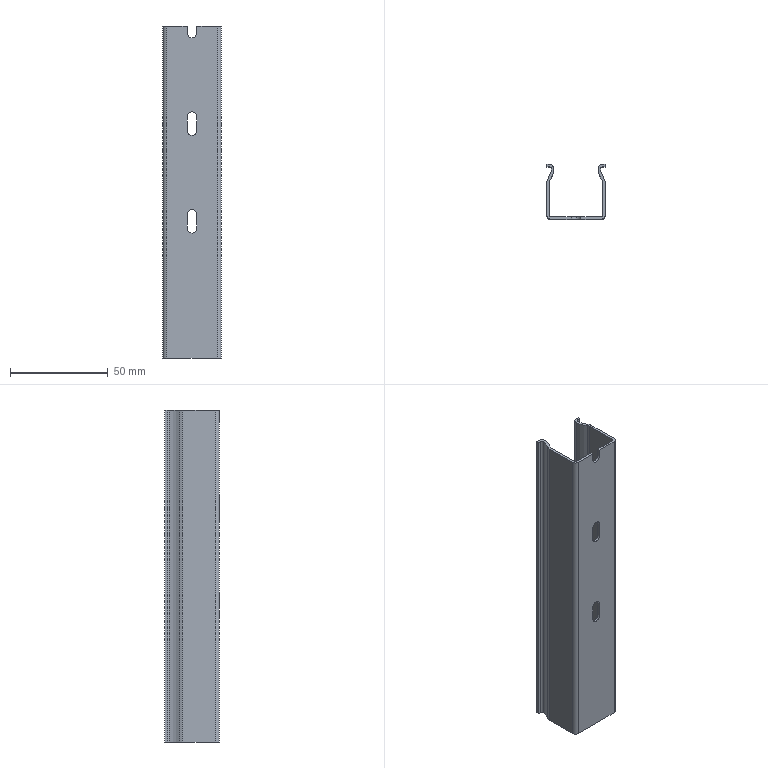Part | SolidWorks | features BaseBody 1 | 1 solid | 47 faces | box 30 x 28 x 170 mm | volume 18284 mm3 | cylinder 26 | plane 21 | commonest cylinder face diameters 5 x8 2 x3 4.5 x3 1.5 x2 3.5 x2 4 x2
STEP:
#1=CARTESIAN_POINT('',(-2.5,-12.75,-103.5));
#2=VERTEX_POINT('',#1);
#3=CARTESIAN_POINT('',(-2.5,-12.75,-96.5));
#4=VERTEX_POINT('',#3);
#5=CARTESIAN_POINT('',(-2.5,-12.75,-96.5));
#6=DIRECTION('',(0.,0.,1.));
#7=VECTOR('',#6,1000.);
#8=LINE('',#5,#7);
#9=EDGE_CURVE('',#2,#4,#8,.T.);
#10=ORIENTED_EDGE('',*,*,#9,.T.);
#11=CARTESIAN_POINT('',(-2.5,-14.,-96.5));
#12=VERTEX_POINT('',#11);
#13=CARTESIAN_POINT('',(-2.5,14.001,-96.5));
#14=DIRECTION('',(0.,-1.,0.));
#15=VECTOR('',#14,1000.);
#16=LINE('',#13,#15);
#17=EDGE_CURVE('',#4,#12,#16,.T.);
#18=ORIENTED_EDGE('',*,*,#17,.T.);
#19=CARTESIAN_POINT('',(-2.5,-14.,-103.5));
#20=VERTEX_POINT('',#19);
#21=CARTESIAN_POINT('',(-2.5,-14.,-96.5));
#22=DIRECTION('',(0.,0.,-1.));
#23=VECTOR('',#22,1000.);
#24=LINE('',#21,#23);
#25=EDGE_CURVE('',#12,#20,#24,.T.);
#26=ORIENTED_EDGE('',*,*,#25,.T.);
#27=CARTESIAN_POINT('',(-2.5,14.001,-103.5));
#28=DIRECTION('',(0.,-1.,0.));
#29=VECTOR('',#28,1000.);
#30=LINE('',#27,#29);
#31=EDGE_CURVE('',#2,#20,#30,.T.);
#32=ORIENTED_EDGE('',*,*,#31,.F.);
#33=EDGE_LOOP('',(#10,#18,#26,#32));
#34=FACE_OUTER_BOUND('',#33,.T.);
#35=CARTESIAN_POINT('',(-2.5,14.001,-96.5));
#36=DIRECTION('',(-1.,0.,0.));
#37=DIRECTION('',(0.,0.,1.));
#38=AXIS2_PLACEMENT_3D('',#35,#36,#37);
#39=PLANE('',#38);
#40=ADVANCED_FACE('',(#34),#39,.F.);
#41=CARTESIAN_POINT('',(0.,-12.75,-106.));
#42=VERTEX_POINT('',#41);
#43=CARTESIAN_POINT('',(0.,-14.,-106.));
#44=VERTEX_POINT('',#43);
#45=CARTESIAN_POINT('',(0.,14.001,-106.));
#46=DIRECTION('',(0.,-1.,0.));
#47=VECTOR('',#46,1000.);
#48=LINE('',#45,#47);
#49=EDGE_CURVE('',#42,#44,#48,.T.);
#50=ORIENTED_EDGE('',*,*,#49,.F.);
#51=CARTESIAN_POINT('',(0.,-12.75,-103.5));
#52=DIRECTION('',(0.,1.,0.));
#53=DIRECTION('',(0.,0.,-1.));
#54=AXIS2_PLACEMENT_3D('',#51,#52,#53);
#55=CIRCLE('',#54,2.5);
#56=EDGE_CURVE('',#42,#2,#55,.T.);
#57=ORIENTED_EDGE('',*,*,#56,.T.);
#58=ORIENTED_EDGE('',*,*,#31,.T.);
#59=CARTESIAN_POINT('',(0.,-14.,-103.5));
#60=DIRECTION('',(0.,-1.,0.));
#61=DIRECTION('',(0.,0.,-1.));
#62=AXIS2_PLACEMENT_3D('',#59,#60,#61);
#63=CIRCLE('',#62,2.5);
#64=EDGE_CURVE('',#20,#44,#63,.T.);
#65=ORIENTED_EDGE('',*,*,#64,.T.);
#66=EDGE_LOOP('',(#50,#57,#58,#65));
#67=FACE_OUTER_BOUND('',#66,.T.);
#68=CARTESIAN_POINT('',(0.,14.001,-103.5));
#69=DIRECTION('',(0.,-1.,0.));
#70=DIRECTION('',(0.,0.,-1.));
#71=AXIS2_PLACEMENT_3D('',#68,#69,#70);
#72=CYLINDRICAL_SURFACE('',#71,2.5);
#73=ADVANCED_FACE('',(#67),#72,.F.);
#74=CARTESIAN_POINT('',(2.5,-12.75,-96.5));
#75=VERTEX_POINT('',#74);
#76=CARTESIAN_POINT('',(2.5,-12.75,-103.5));
#77=VERTEX_POINT('',#76);
#78=CARTESIAN_POINT('',(2.5,-12.75,-96.5));
#79=DIRECTION('',(0.,0.,-1.));
#80=VECTOR('',#79,1000.);
#81=LINE('',#78,#80);
#82=EDGE_CURVE('',#75,#77,#81,.T.);
#83=ORIENTED_EDGE('',*,*,#82,.T.);
#84=CARTESIAN_POINT('',(2.5,-14.,-103.5));
#85=VERTEX_POINT('',#84);
#86=CARTESIAN_POINT('',(2.5,14.001,-103.5));
#87=DIRECTION('',(0.,-1.,0.));
#88=VECTOR('',#87,1000.);
#89=LINE('',#86,#88);
#90=EDGE_CURVE('',#77,#85,#89,.T.);
#91=ORIENTED_EDGE('',*,*,#90,.T.);
#92=CARTESIAN_POINT('',(2.5,-14.,-96.5));
#93=VERTEX_POINT('',#92);
#94=CARTESIAN_POINT('',(2.5,-14.,-96.5));
#95=DIRECTION('',(0.,0.,1.));
#96=VECTOR('',#95,1000.);
#97=LINE('',#94,#96);
#98=EDGE_CURVE('',#85,#93,#97,.T.);
#99=ORIENTED_EDGE('',*,*,#98,.T.);
#100=CARTESIAN_POINT('',(2.5,14.001,-96.5));
#101=DIRECTION('',(0.,-1.,0.));
#102=VECTOR('',#101,1000.);
#103=LINE('',#100,#102);
#104=EDGE_CURVE('',#75,#93,#103,.T.);
#105=ORIENTED_EDGE('',*,*,#104,.F.);
#106=EDGE_LOOP('',(#83,#91,#99,#105));
#107=FACE_OUTER_BOUND('',#106,.T.);
#108=CARTESIAN_POINT('',(2.5,14.001,-96.5));
#109=DIRECTION('',(1.,0.,0.));
#110=DIRECTION('',(0.,0.,1.));
#111=AXIS2_PLACEMENT_3D('',#108,#109,#110);
#112=PLANE('',#111);
#113=ADVANCED_FACE('',(#107),#112,.F.);
#114=CARTESIAN_POINT('',(0.,-12.75,-96.5));
#115=DIRECTION('',(0.,1.,0.));
#116=DIRECTION('',(0.,0.,-1.));
#117=AXIS2_PLACEMENT_3D('',#114,#115,#116);
#118=CIRCLE('',#117,2.5);
#119=EDGE_CURVE('',#4,#75,#118,.T.);
#120=ORIENTED_EDGE('',*,*,#119,.T.);
#121=ORIENTED_EDGE('',*,*,#104,.T.);
#122=CARTESIAN_POINT('',(0.,-14.,-96.5));
#123=DIRECTION('',(0.,-1.,0.));
#124=DIRECTION('',(0.,0.,-1.));
#125=AXIS2_PLACEMENT_3D('',#122,#123,#124);
#126=CIRCLE('',#125,2.5);
#127=EDGE_CURVE('',#93,#12,#126,.T.);
#128=ORIENTED_EDGE('',*,*,#127,.T.);
#129=ORIENTED_EDGE('',*,*,#17,.F.);
#130=EDGE_LOOP('',(#120,#121,#128,#129));
#131=FACE_OUTER_BOUND('',#130,.T.);
#132=CARTESIAN_POINT('',(0.,14.001,-96.5));
#133=DIRECTION('',(0.,-1.,0.));
#134=DIRECTION('',(0.,0.,-1.));
#135=AXIS2_PLACEMENT_3D('',#132,#133,#134);
#136=CYLINDRICAL_SURFACE('',#135,2.5);
#137=ADVANCED_FACE('',(#131),#136,.F.);
#138=CARTESIAN_POINT('',(-2.5,-12.75,-53.5));
#139=VERTEX_POINT('',#138);
#140=CARTESIAN_POINT('',(-2.5,-12.75,-46.5));
#141=VERTEX_POINT('',#140);
#142=CARTESIAN_POINT('',(-2.5,-12.75,-46.5));
#143=DIRECTION('',(0.,0.,1.));
#144=VECTOR('',#143,1000.);
#145=LINE('',#142,#144);
#146=EDGE_CURVE('',#139,#141,#145,.T.);
#147=ORIENTED_EDGE('',*,*,#146,.T.);
#148=CARTESIAN_POINT('',(-2.5,-14.,-46.5));
#149=VERTEX_POINT('',#148);
#150=CARTESIAN_POINT('',(-2.5,14.001,-46.5));
#151=DIRECTION('',(0.,-1.,0.));
#152=VECTOR('',#151,1000.);
#153=LINE('',#150,#152);
#154=EDGE_CURVE('',#141,#149,#153,.T.);
#155=ORIENTED_EDGE('',*,*,#154,.T.);
#156=CARTESIAN_POINT('',(-2.5,-14.,-53.5));
#157=VERTEX_POINT('',#156);
#158=CARTESIAN_POINT('',(-2.5,-14.,-46.5));
#159=DIRECTION('',(0.,0.,-1.));
#160=VECTOR('',#159,1000.);
#161=LINE('',#158,#160);
#162=EDGE_CURVE('',#149,#157,#161,.T.);
#163=ORIENTED_EDGE('',*,*,#162,.T.);
#164=CARTESIAN_POINT('',(-2.5,14.001,-53.5));
#165=DIRECTION('',(0.,-1.,0.));
#166=VECTOR('',#165,1000.);
#167=LINE('',#164,#166);
#168=EDGE_CURVE('',#139,#157,#167,.T.);
#169=ORIENTED_EDGE('',*,*,#168,.F.);
#170=EDGE_LOOP('',(#147,#155,#163,#169));
#171=FACE_OUTER_BOUND('',#170,.T.);
#172=CARTESIAN_POINT('',(-2.5,14.001,-46.5));
#173=DIRECTION('',(-1.,0.,0.));
#174=DIRECTION('',(0.,0.,1.));
#175=AXIS2_PLACEMENT_3D('',#172,#173,#174);
#176=PLANE('',#175);
#177=ADVANCED_FACE('',(#171),#176,.F.);
#178=CARTESIAN_POINT('',(0.,-12.75,-56.));
#179=VERTEX_POINT('',#178);
#180=CARTESIAN_POINT('',(0.,-14.,-56.));
#181=VERTEX_POINT('',#180);
#182=CARTESIAN_POINT('',(0.,14.001,-56.));
#183=DIRECTION('',(0.,-1.,0.));
#184=VECTOR('',#183,1000.);
#185=LINE('',#182,#184);
#186=EDGE_CURVE('',#179,#181,#185,.T.);
#187=ORIENTED_EDGE('',*,*,#186,.F.);
#188=CARTESIAN_POINT('',(0.,-12.75,-53.5));
#189=DIRECTION('',(0.,1.,0.));
#190=DIRECTION('',(0.,0.,-1.));
#191=AXIS2_PLACEMENT_3D('',#188,#189,#190);
#192=CIRCLE('',#191,2.5);
#193=EDGE_CURVE('',#179,#139,#192,.T.);
#194=ORIENTED_EDGE('',*,*,#193,.T.);
#195=ORIENTED_EDGE('',*,*,#168,.T.);
#196=CARTESIAN_POINT('',(0.,-14.,-53.5));
#197=DIRECTION('',(0.,-1.,0.));
#198=DIRECTION('',(0.,0.,-1.));
#199=AXIS2_PLACEMENT_3D('',#196,#197,#198);
#200=CIRCLE('',#199,2.5);
#201=EDGE_CURVE('',#157,#181,#200,.T.);
#202=ORIENTED_EDGE('',*,*,#201,.T.);
#203=EDGE_LOOP('',(#187,#194,#195,#202));
#204=FACE_OUTER_BOUND('',#203,.T.);
#205=CARTESIAN_POINT('',(0.,14.001,-53.5));
#206=DIRECTION('',(0.,-1.,0.));
#207=DIRECTION('',(0.,0.,-1.));
#208=AXIS2_PLACEMENT_3D('',#205,#206,#207);
#209=CYLINDRICAL_SURFACE('',#208,2.5);
#210=ADVANCED_FACE('',(#204),#209,.F.);
#211=CARTESIAN_POINT('',(2.5,-12.75,-46.5));
#212=VERTEX_POINT('',#211);
#213=CARTESIAN_POINT('',(2.5,-12.75,-53.5));
#214=VERTEX_POINT('',#213);
#215=CARTESIAN_POINT('',(2.5,-12.75,-46.5));
#216=DIRECTION('',(0.,0.,-1.));
#217=VECTOR('',#216,1000.);
#218=LINE('',#215,#217);
#219=EDGE_CURVE('',#212,#214,#218,.T.);
#220=ORIENTED_EDGE('',*,*,#219,.T.);
#221=CARTESIAN_POINT('',(2.5,-14.,-53.5));
#222=VERTEX_POINT('',#221);
#223=CARTESIAN_POINT('',(2.5,14.001,-53.5));
#224=DIRECTION('',(0.,-1.,0.));
#225=VECTOR('',#224,1000.);
#226=LINE('',#223,#225);
#227=EDGE_CURVE('',#214,#222,#226,.T.);
#228=ORIENTED_EDGE('',*,*,#227,.T.);
#229=CARTESIAN_POINT('',(2.5,-14.,-46.5));
#230=VERTEX_POINT('',#229);
#231=CARTESIAN_POINT('',(2.5,-14.,-46.5));
#232=DIRECTION('',(0.,0.,1.));
#233=VECTOR('',#232,1000.);
#234=LINE('',#231,#233);
#235=EDGE_CURVE('',#222,#230,#234,.T.);
#236=ORIENTED_EDGE('',*,*,#235,.T.);
#237=CARTESIAN_POINT('',(2.5,14.001,-46.5));
#238=DIRECTION('',(0.,-1.,0.));
#239=VECTOR('',#238,1000.);
#240=LINE('',#237,#239);
#241=EDGE_CURVE('',#212,#230,#240,.T.);
#242=ORIENTED_EDGE('',*,*,#241,.F.);
#243=EDGE_LOOP('',(#220,#228,#236,#242));
#244=FACE_OUTER_BOUND('',#243,.T.);
#245=CARTESIAN_POINT('',(2.5,14.001,-46.5));
#246=DIRECTION('',(1.,0.,0.));
#247=DIRECTION('',(0.,0.,1.));
#248=AXIS2_PLACEMENT_3D('',#245,#246,#247);
#249=PLANE('',#248);
#250=ADVANCED_FACE('',(#244),#249,.F.);
#251=CARTESIAN_POINT('',(0.,-12.75,-46.5));
#252=DIRECTION('',(0.,1.,0.));
#253=DIRECTION('',(0.,0.,-1.));
#254=AXIS2_PLACEMENT_3D('',#251,#252,#253);
#255=CIRCLE('',#254,2.5);
#256=EDGE_CURVE('',#141,#212,#255,.T.);
#257=ORIENTED_EDGE('',*,*,#256,.T.);
#258=ORIENTED_EDGE('',*,*,#241,.T.);
#259=CARTESIAN_POINT('',(0.,-14.,-46.5));
#260=DIRECTION('',(0.,-1.,0.));
#261=DIRECTION('',(0.,0.,-1.));
#262=AXIS2_PLACEMENT_3D('',#259,#260,#261);
#263=CIRCLE('',#262,2.5);
#264=EDGE_CURVE('',#230,#149,#263,.T.);
#265=ORIENTED_EDGE('',*,*,#264,.T.);
#266=ORIENTED_EDGE('',*,*,#154,.F.);
#267=EDGE_LOOP('',(#257,#258,#265,#266));
#268=FACE_OUTER_BOUND('',#267,.T.);
#269=CARTESIAN_POINT('',(0.,14.001,-46.5));
#270=DIRECTION('',(0.,-1.,0.));
#271=DIRECTION('',(0.,0.,-1.));
#272=AXIS2_PLACEMENT_3D('',#269,#270,#271);
#273=CYLINDRICAL_SURFACE('',#272,2.5);
#274=ADVANCED_FACE('',(#268),#273,.F.);
#275=CARTESIAN_POINT('',(-2.5,-14.,0.));
#276=VERTEX_POINT('',#275);
#277=CARTESIAN_POINT('',(-2.5,-14.,-3.5));
#278=VERTEX_POINT('',#277);
#279=CARTESIAN_POINT('',(-2.5,-14.,3.5));
#280=DIRECTION('',(0.,0.,-1.));
#281=VECTOR('',#280,1000.);
#282=LINE('',#279,#281);
#283=EDGE_CURVE('',#276,#278,#282,.T.);
#284=ORIENTED_EDGE('',*,*,#283,.T.);
#285=CARTESIAN_POINT('',(-2.5,-12.75,-3.5));
#286=VERTEX_POINT('',#285);
#287=CARTESIAN_POINT('',(-2.5,14.001,-3.5));
#288=DIRECTION('',(0.,-1.,0.));
#289=VECTOR('',#288,1000.);
#290=LINE('',#287,#289);
#291=EDGE_CURVE('',#286,#278,#290,.T.);
#292=ORIENTED_EDGE('',*,*,#291,.F.);
#293=CARTESIAN_POINT('',(-2.5,-12.75,0.));
#294=VERTEX_POINT('',#293);
#295=CARTESIAN_POINT('',(-2.5,-12.75,3.5));
#296=DIRECTION('',(0.,0.,1.));
#297=VECTOR('',#296,1000.);
#298=LINE('',#295,#297);
#299=EDGE_CURVE('',#286,#294,#298,.T.);
#300=ORIENTED_EDGE('',*,*,#299,.T.);
#301=CARTESIAN_POINT('',(-2.5,14.001,0.));
#302=DIRECTION('',(0.,1.,0.));
#303=VECTOR('',#302,1000.);
#304=LINE('',#301,#303);
#305=EDGE_CURVE('',#276,#294,#304,.T.);
#306=ORIENTED_EDGE('',*,*,#305,.F.);
#307=EDGE_LOOP('',(#284,#292,#300,#306));
#308=FACE_OUTER_BOUND('',#307,.T.);
#309=CARTESIAN_POINT('',(-2.5,14.001,3.5));
#310=DIRECTION('',(-1.,0.,0.));
#311=DIRECTION('',(0.,0.,1.));
#312=AXIS2_PLACEMENT_3D('',#309,#310,#311);
#313=PLANE('',#312);
#314=ADVANCED_FACE('',(#308),#313,.F.);
#315=CARTESIAN_POINT('',(2.5,-12.75,0.));
#316=VERTEX_POINT('',#315);
#317=CARTESIAN_POINT('',(2.5,-12.75,-3.5));
#318=VERTEX_POINT('',#317);
#319=CARTESIAN_POINT('',(2.5,-12.75,3.5));
#320=DIRECTION('',(0.,0.,-1.));
#321=VECTOR('',#320,1000.);
#322=LINE('',#319,#321);
#323=EDGE_CURVE('',#316,#318,#322,.T.);
#324=ORIENTED_EDGE('',*,*,#323,.T.);
#325=CARTESIAN_POINT('',(2.5,-14.,-3.5));
#326=VERTEX_POINT('',#325);
#327=CARTESIAN_POINT('',(2.5,14.001,-3.5));
#328=DIRECTION('',(0.,-1.,0.));
#329=VECTOR('',#328,1000.);
#330=LINE('',#327,#329);
#331=EDGE_CURVE('',#318,#326,#330,.T.);
#332=ORIENTED_EDGE('',*,*,#331,.T.);
#333=CARTESIAN_POINT('',(2.5,-14.,0.));
#334=VERTEX_POINT('',#333);
#335=CARTESIAN_POINT('',(2.5,-14.,3.5));
#336=DIRECTION('',(0.,0.,1.));
#337=VECTOR('',#336,1000.);
#338=LINE('',#335,#337);
#339=EDGE_CURVE('',#326,#334,#338,.T.);
#340=ORIENTED_EDGE('',*,*,#339,.T.);
#341=CARTESIAN_POINT('',(2.5,14.001,0.));
#342=DIRECTION('',(0.,-1.,0.));
#343=VECTOR('',#342,1000.);
#344=LINE('',#341,#343);
#345=EDGE_CURVE('',#316,#334,#344,.T.);
#346=ORIENTED_EDGE('',*,*,#345,.F.);
#347=EDGE_LOOP('',(#324,#332,#340,#346));
#348=FACE_OUTER_BOUND('',#347,.T.);
#349=CARTESIAN_POINT('',(2.5,14.001,3.5));
#350=DIRECTION('',(1.,0.,0.));
#351=DIRECTION('',(0.,0.,1.));
#352=AXIS2_PLACEMENT_3D('',#349,#350,#351);
#353=PLANE('',#352);
#354=ADVANCED_FACE('',(#348),#353,.F.);
#355=CARTESIAN_POINT('',(0.,-12.75,-6.));
#356=VERTEX_POINT('',#355);
#357=CARTESIAN_POINT('',(0.,-14.,-6.));
#358=VERTEX_POINT('',#357);
#359=CARTESIAN_POINT('',(0.,14.001,-6.));
#360=DIRECTION('',(0.,-1.,0.));
#361=VECTOR('',#360,1000.);
#362=LINE('',#359,#361);
#363=EDGE_CURVE('',#356,#358,#362,.T.);
#364=ORIENTED_EDGE('',*,*,#363,.F.);
#365=CARTESIAN_POINT('',(0.,-12.75,-3.5));
#366=DIRECTION('',(0.,1.,0.));
#367=DIRECTION('',(0.,0.,-1.));
#368=AXIS2_PLACEMENT_3D('',#365,#366,#367);
#369=CIRCLE('',#368,2.5);
#370=EDGE_CURVE('',#356,#286,#369,.T.);
#371=ORIENTED_EDGE('',*,*,#370,.T.);
#372=ORIENTED_EDGE('',*,*,#291,.T.);
#373=CARTESIAN_POINT('',(0.,-14.,-3.5));
#374=DIRECTION('',(0.,-1.,0.));
#375=DIRECTION('',(0.,0.,-1.));
#376=AXIS2_PLACEMENT_3D('',#373,#374,#375);
#377=CIRCLE('',#376,2.5);
#378=EDGE_CURVE('',#278,#358,#377,.T.);
#379=ORIENTED_EDGE('',*,*,#378,.T.);
#380=EDGE_LOOP('',(#364,#371,#372,#379));
#381=FACE_OUTER_BOUND('',#380,.T.);
#382=CARTESIAN_POINT('',(0.,14.001,-3.5));
#383=DIRECTION('',(0.,-1.,0.));
#384=DIRECTION('',(0.,0.,-1.));
#385=AXIS2_PLACEMENT_3D('',#382,#383,#384);
#386=CYLINDRICAL_SURFACE('',#385,2.5);
#387=ADVANCED_FACE('',(#381),#386,.F.);
#388=CARTESIAN_POINT('',(-13.,-12.75,-170.));
#389=VERTEX_POINT('',#388);
#390=CARTESIAN_POINT('',(-13.75,-12.,-170.));
#391=VERTEX_POINT('',#390);
#392=CARTESIAN_POINT('',(-13.,-12.,-170.));
#393=DIRECTION('',(0.,0.,-1.));
#394=DIRECTION('',(1.,0.,0.));
#395=AXIS2_PLACEMENT_3D('',#392,#393,#394);
#396=CIRCLE('',#395,0.75);
#397=EDGE_CURVE('',#389,#391,#396,.T.);
#398=ORIENTED_EDGE('',*,*,#397,.T.);
#399=CARTESIAN_POINT('',(-13.75,-12.,0.));
#400=VERTEX_POINT('',#399);
#401=CARTESIAN_POINT('',(-13.75,-12.,-170.));
#402=DIRECTION('',(0.,0.,1.));
#403=VECTOR('',#402,1000.);
#404=LINE('',#401,#403);
#405=EDGE_CURVE('',#391,#400,#404,.T.);
#406=ORIENTED_EDGE('',*,*,#405,.T.);
#407=CARTESIAN_POINT('',(-13.,-12.75,0.));
#408=VERTEX_POINT('',#407);
#409=CARTESIAN_POINT('',(-13.,-12.,0.));
#410=DIRECTION('',(0.,0.,1.));
#411=DIRECTION('',(1.,0.,0.));
#412=AXIS2_PLACEMENT_3D('',#409,#410,#411);
#413=CIRCLE('',#412,0.75);
#414=EDGE_CURVE('',#400,#408,#413,.T.);
#415=ORIENTED_EDGE('',*,*,#414,.T.);
#416=CARTESIAN_POINT('',(-13.,-12.75,-170.));
#417=DIRECTION('',(0.,0.,-1.));
#418=VECTOR('',#417,1000.);
#419=LINE('',#416,#418);
#420=EDGE_CURVE('',#408,#389,#419,.T.);
#421=ORIENTED_EDGE('',*,*,#420,.T.);
#422=EDGE_LOOP('',(#398,#406,#415,#421));
#423=FACE_OUTER_BOUND('',#422,.T.);
#424=CARTESIAN_POINT('',(-13.,-12.,-170.));
#425=DIRECTION('',(0.,0.,1.));
#426=DIRECTION('',(1.,0.,0.));
#427=AXIS2_PLACEMENT_3D('',#424,#425,#426);
#428=CYLINDRICAL_SURFACE('',#427,0.75);
#429=ADVANCED_FACE('',(#423),#428,.F.);
#430=CARTESIAN_POINT('',(13.75,-12.,-170.));
#431=VERTEX_POINT('',#430);
#432=CARTESIAN_POINT('',(13.,-12.75,-170.));
#433=VERTEX_POINT('',#432);
#434=CARTESIAN_POINT('',(13.,-12.,-170.));
#435=DIRECTION('',(0.,0.,-1.));
#436=DIRECTION('',(1.,0.,0.));
#437=AXIS2_PLACEMENT_3D('',#434,#435,#436);
#438=CIRCLE('',#437,0.75);
#439=EDGE_CURVE('',#431,#433,#438,.T.);
#440=ORIENTED_EDGE('',*,*,#439,.T.);
#441=CARTESIAN_POINT('',(13.,-12.75,0.));
#442=VERTEX_POINT('',#441);
#443=CARTESIAN_POINT('',(13.,-12.75,-170.));
#444=DIRECTION('',(0.,0.,1.));
#445=VECTOR('',#444,1000.);
#446=LINE('',#443,#445);
#447=EDGE_CURVE('',#433,#442,#446,.T.);
#448=ORIENTED_EDGE('',*,*,#447,.T.);
#449=CARTESIAN_POINT('',(13.75,-12.,0.));
#450=VERTEX_POINT('',#449);
#451=CARTESIAN_POINT('',(13.,-12.,0.));
#452=DIRECTION('',(0.,0.,1.));
#453=DIRECTION('',(1.,0.,0.));
#454=AXIS2_PLACEMENT_3D('',#451,#452,#453);
#455=CIRCLE('',#454,0.75);
#456=EDGE_CURVE('',#442,#450,#455,.T.);
#457=ORIENTED_EDGE('',*,*,#456,.T.);
#458=CARTESIAN_POINT('',(13.75,-12.,-170.));
#459=DIRECTION('',(0.,0.,-1.));
#460=VECTOR('',#459,1000.);
#461=LINE('',#458,#460);
#462=EDGE_CURVE('',#450,#431,#461,.T.);
#463=ORIENTED_EDGE('',*,*,#462,.T.);
#464=EDGE_LOOP('',(#440,#448,#457,#463));
#465=FACE_OUTER_BOUND('',#464,.T.);
#466=CARTESIAN_POINT('',(13.,-12.,-170.));
#467=DIRECTION('',(0.,0.,1.));
#468=DIRECTION('',(1.,0.,0.));
#469=AXIS2_PLACEMENT_3D('',#466,#467,#468);
#470=CYLINDRICAL_SURFACE('',#469,0.75);
#471=ADVANCED_FACE('',(#465),#470,.F.);
#472=CARTESIAN_POINT('',(13.439,5.746,-170.));
#473=VERTEX_POINT('',#472);
#474=CARTESIAN_POINT('',(13.75,4.75,-170.));
#475=VERTEX_POINT('',#474);
#476=CARTESIAN_POINT('',(12.,4.75,-170.));
#477=DIRECTION('',(0.,0.,-1.));
#478=DIRECTION('',(1.,0.,0.));
#479=AXIS2_PLACEMENT_3D('',#476,#477,#478);
#480=CIRCLE('',#479,1.75);
#481=EDGE_CURVE('',#473,#475,#480,.T.);
#482=ORIENTED_EDGE('',*,*,#481,.T.);
#483=CARTESIAN_POINT('',(13.75,4.75,0.));
#484=VERTEX_POINT('',#483);
#485=CARTESIAN_POINT('',(13.75,4.75,-170.));
#486=DIRECTION('',(0.,0.,1.));
#487=VECTOR('',#486,1000.);
#488=LINE('',#485,#487);
#489=EDGE_CURVE('',#475,#484,#488,.T.);
#490=ORIENTED_EDGE('',*,*,#489,.T.);
#491=CARTESIAN_POINT('',(13.439,5.746,0.));
#492=VERTEX_POINT('',#491);
#493=CARTESIAN_POINT('',(12.,4.75,0.));
#494=DIRECTION('',(0.,0.,1.));
#495=DIRECTION('',(1.,0.,0.));
#496=AXIS2_PLACEMENT_3D('',#493,#494,#495);
#497=CIRCLE('',#496,1.75);
#498=EDGE_CURVE('',#484,#492,#497,.T.);
#499=ORIENTED_EDGE('',*,*,#498,.T.);
#500=CARTESIAN_POINT('',(13.439,5.746,-170.));
#501=DIRECTION('',(0.,0.,-1.));
#502=VECTOR('',#501,1000.);
#503=LINE('',#500,#502);
#504=EDGE_CURVE('',#492,#473,#503,.T.);
#505=ORIENTED_EDGE('',*,*,#504,.T.);
#506=EDGE_LOOP('',(#482,#490,#499,#505));
#507=FACE_OUTER_BOUND('',#506,.T.);
#508=CARTESIAN_POINT('',(12.,4.75,-170.));
#509=DIRECTION('',(0.,0.,1.));
#510=DIRECTION('',(1.,0.,0.));
#511=AXIS2_PLACEMENT_3D('',#508,#509,#510);
#512=CYLINDRICAL_SURFACE('',#511,1.75);
#513=ADVANCED_FACE('',(#507),#512,.F.);
#514=CARTESIAN_POINT('',(-13.75,4.75,-170.));
#515=VERTEX_POINT('',#514);
#516=CARTESIAN_POINT('',(-13.439,5.746,-170.));
#517=VERTEX_POINT('',#516);
#518=CARTESIAN_POINT('',(-12.,4.75,-170.));
#519=DIRECTION('',(0.,0.,-1.));
#520=DIRECTION('',(1.,0.,0.));
#521=AXIS2_PLACEMENT_3D('',#518,#519,#520);
#522=CIRCLE('',#521,1.75);
#523=EDGE_CURVE('',#515,#517,#522,.T.);
#524=ORIENTED_EDGE('',*,*,#523,.T.);
#525=CARTESIAN_POINT('',(-13.439,5.746,0.));
#526=VERTEX_POINT('',#525);
#527=CARTESIAN_POINT('',(-13.439,5.746,-170.));
#528=DIRECTION('',(0.,0.,1.));
#529=VECTOR('',#528,1000.);
#530=LINE('',#527,#529);
#531=EDGE_CURVE('',#517,#526,#530,.T.);
#532=ORIENTED_EDGE('',*,*,#531,.T.);
#533=CARTESIAN_POINT('',(-13.75,4.75,0.));
#534=VERTEX_POINT('',#533);
#535=CARTESIAN_POINT('',(-12.,4.75,0.));
#536=DIRECTION('',(0.,0.,1.));
#537=DIRECTION('',(1.,0.,0.));
#538=AXIS2_PLACEMENT_3D('',#535,#536,#537);
#539=CIRCLE('',#538,1.75);
#540=EDGE_CURVE('',#526,#534,#539,.T.);
#541=ORIENTED_EDGE('',*,*,#540,.T.);
#542=CARTESIAN_POINT('',(-13.75,4.75,-170.));
#543=DIRECTION('',(0.,0.,-1.));
#544=VECTOR('',#543,1000.);
#545=LINE('',#542,#544);
#546=EDGE_CURVE('',#534,#515,#545,.T.);
#547=ORIENTED_EDGE('',*,*,#546,.T.);
#548=EDGE_LOOP('',(#524,#532,#541,#547));
#549=FACE_OUTER_BOUND('',#548,.T.);
#550=CARTESIAN_POINT('',(-12.,4.75,-170.));
#551=DIRECTION('',(0.,0.,1.));
#552=DIRECTION('',(1.,0.,0.));
#553=AXIS2_PLACEMENT_3D('',#550,#551,#552);
#554=CYLINDRICAL_SURFACE('',#553,1.75);
#555=ADVANCED_FACE('',(#549),#554,.F.);
#556=CARTESIAN_POINT('',(13.55,14.,-170.));
#557=VERTEX_POINT('',#556);
#558=CARTESIAN_POINT('',(11.311,11.526,-170.));
#559=VERTEX_POINT('',#558);
#560=CARTESIAN_POINT('',(13.55,11.75,-170.));
#561=DIRECTION('',(0.,0.,1.));
#562=DIRECTION('',(1.,0.,0.));
#563=AXIS2_PLACEMENT_3D('',#560,#561,#562);
#564=CIRCLE('',#563,2.25);
#565=EDGE_CURVE('',#557,#559,#564,.T.);
#566=ORIENTED_EDGE('',*,*,#565,.T.);
#567=CARTESIAN_POINT('',(11.311,11.526,0.));
#568=VERTEX_POINT('',#567);
#569=CARTESIAN_POINT('',(11.311,11.526,-170.));
#570=DIRECTION('',(0.,0.,1.));
#571=VECTOR('',#570,1000.);
#572=LINE('',#569,#571);
#573=EDGE_CURVE('',#559,#568,#572,.T.);
#574=ORIENTED_EDGE('',*,*,#573,.T.);
#575=CARTESIAN_POINT('',(13.55,14.,0.));
#576=VERTEX_POINT('',#575);
#577=CARTESIAN_POINT('',(13.55,11.75,0.));
#578=DIRECTION('',(0.,0.,-1.));
#579=DIRECTION('',(1.,0.,0.));
#580=AXIS2_PLACEMENT_3D('',#577,#578,#579);
#581=CIRCLE('',#580,2.25);
#582=EDGE_CURVE('',#568,#576,#581,.T.);
#583=ORIENTED_EDGE('',*,*,#582,.T.);
#584=CARTESIAN_POINT('',(13.55,14.,-170.));
#585=DIRECTION('',(0.,0.,-1.));
#586=VECTOR('',#585,1000.);
#587=LINE('',#584,#586);
#588=EDGE_CURVE('',#576,#557,#587,.T.);
#589=ORIENTED_EDGE('',*,*,#588,.T.);
#590=EDGE_LOOP('',(#566,#574,#583,#589));
#591=FACE_OUTER_BOUND('',#590,.T.);
#592=CARTESIAN_POINT('',(13.55,11.75,-170.));
#593=DIRECTION('',(0.,0.,1.));
#594=DIRECTION('',(1.,0.,0.));
#595=AXIS2_PLACEMENT_3D('',#592,#593,#594);
#596=CYLINDRICAL_SURFACE('',#595,2.25);
#597=ADVANCED_FACE('',(#591),#596,.T.);
#598=CARTESIAN_POINT('',(-11.3,11.75,-170.));
#599=VERTEX_POINT('',#598);
#600=CARTESIAN_POINT('',(-11.3,11.75,0.));
#601=VERTEX_POINT('',#600);
#602=CARTESIAN_POINT('',(-11.3,11.75,-170.));
#603=DIRECTION('',(0.,0.,1.));
#604=VECTOR('',#603,1000.);
#605=LINE('',#602,#604);
#606=EDGE_CURVE('',#599,#601,#605,.T.);
#607=ORIENTED_EDGE('',*,*,#606,.F.);
#608=CARTESIAN_POINT('',(-13.55,14.,-170.));
#609=VERTEX_POINT('',#608);
#610=CARTESIAN_POINT('',(-13.55,11.75,-170.));
#611=DIRECTION('',(0.,0.,1.));
#612=DIRECTION('',(1.,0.,0.));
#613=AXIS2_PLACEMENT_3D('',#610,#611,#612);
#614=CIRCLE('',#613,2.25);
#615=EDGE_CURVE('',#599,#609,#614,.T.);
#616=ORIENTED_EDGE('',*,*,#615,.T.);
#617=CARTESIAN_POINT('',(-13.55,14.,0.));
#618=VERTEX_POINT('',#617);
#619=CARTESIAN_POINT('',(-13.55,14.,-170.));
#620=DIRECTION('',(0.,0.,1.));
#621=VECTOR('',#620,1000.);
#622=LINE('',#619,#621);
#623=EDGE_CURVE('',#609,#618,#622,.T.);
#624=ORIENTED_EDGE('',*,*,#623,.T.);
#625=CARTESIAN_POINT('',(-13.55,11.75,0.));
#626=DIRECTION('',(0.,0.,-1.));
#627=DIRECTION('',(1.,0.,0.));
#628=AXIS2_PLACEMENT_3D('',#625,#626,#627);
#629=CIRCLE('',#628,2.25);
#630=EDGE_CURVE('',#618,#601,#629,.T.);
#631=ORIENTED_EDGE('',*,*,#630,.T.);
#632=EDGE_LOOP('',(#607,#616,#624,#631));
#633=FACE_OUTER_BOUND('',#632,.T.);
#634=CARTESIAN_POINT('',(-13.55,11.75,-170.));
#635=DIRECTION('',(0.,0.,1.));
#636=DIRECTION('',(1.,0.,0.));
#637=AXIS2_PLACEMENT_3D('',#634,#635,#636);
#638=CYLINDRICAL_SURFACE('',#637,2.25);
#639=ADVANCED_FACE('',(#633),#638,.T.);
#640=CARTESIAN_POINT('',(-11.311,11.526,-170.));
#641=VERTEX_POINT('',#640);
#642=CARTESIAN_POINT('',(-23.55,12.75,-170.));
#643=DIRECTION('',(0.,0.,1.));
#644=DIRECTION('',(1.,0.,0.));
#645=AXIS2_PLACEMENT_3D('',#642,#643,#644);
#646=CIRCLE('',#645,12.3);
#647=EDGE_CURVE('',#517,#641,#646,.T.);
#648=ORIENTED_EDGE('',*,*,#647,.T.);
#649=CARTESIAN_POINT('',(-11.311,11.526,0.));
#650=VERTEX_POINT('',#649);
#651=CARTESIAN_POINT('',(-11.311,11.526,-170.));
#652=DIRECTION('',(0.,0.,-1.));
#653=VECTOR('',#652,1000.);
#654=LINE('',#651,#653);
#655=EDGE_CURVE('',#650,#641,#654,.T.);
#656=ORIENTED_EDGE('',*,*,#655,.F.);
#657=CARTESIAN_POINT('',(-23.55,12.75,0.));
#658=DIRECTION('',(0.,0.,1.));
#659=DIRECTION('',(1.,0.,0.));
#660=AXIS2_PLACEMENT_3D('',#657,#658,#659);
#661=CIRCLE('',#660,12.3);
#662=EDGE_CURVE('',#526,#650,#661,.T.);
#663=ORIENTED_EDGE('',*,*,#662,.F.);
#664=ORIENTED_EDGE('',*,*,#531,.F.);
#665=EDGE_LOOP('',(#648,#656,#663,#664));
#666=FACE_OUTER_BOUND('',#665,.T.);
#667=CARTESIAN_POINT('',(-23.55,12.75,-170.));
#668=DIRECTION('',(0.,0.,1.));
#669=DIRECTION('',(1.,0.,0.));
#670=AXIS2_PLACEMENT_3D('',#667,#668,#669);
#671=CYLINDRICAL_SURFACE('',#670,12.3);
#672=ADVANCED_FACE('',(#666),#671,.T.);
#673=CARTESIAN_POINT('',(23.55,12.75,0.));
#674=DIRECTION('',(0.,0.,1.));
#675=DIRECTION('',(1.,0.,0.));
#676=AXIS2_PLACEMENT_3D('',#673,#674,#675);
#677=CIRCLE('',#676,12.3);
#678=EDGE_CURVE('',#568,#492,#677,.T.);
#679=ORIENTED_EDGE('',*,*,#678,.F.);
#680=ORIENTED_EDGE('',*,*,#573,.F.);
#681=CARTESIAN_POINT('',(23.55,12.75,-170.));
#682=DIRECTION('',(0.,0.,1.));
#683=DIRECTION('',(1.,0.,0.));
#684=AXIS2_PLACEMENT_3D('',#681,#682,#683);
#685=CIRCLE('',#684,12.3);
#686=EDGE_CURVE('',#559,#473,#685,.T.);
#687=ORIENTED_EDGE('',*,*,#686,.T.);
#688=ORIENTED_EDGE('',*,*,#504,.F.);
#689=EDGE_LOOP('',(#679,#680,#687,#688));
#690=FACE_OUTER_BOUND('',#689,.T.);
#691=CARTESIAN_POINT('',(23.55,12.75,-170.));
#692=DIRECTION('',(0.,0.,1.));
#693=DIRECTION('',(1.,0.,0.));
#694=AXIS2_PLACEMENT_3D('',#691,#692,#693);
#695=CYLINDRICAL_SURFACE('',#694,12.3);
#696=ADVANCED_FACE('',(#690),#695,.T.);
#697=ORIENTED_EDGE('',*,*,#219,.F.);
#698=ORIENTED_EDGE('',*,*,#256,.F.);
#699=ORIENTED_EDGE('',*,*,#146,.F.);
#700=ORIENTED_EDGE('',*,*,#193,.F.);
#701=CARTESIAN_POINT('',(0.,-12.75,-53.5));
#702=DIRECTION('',(0.,1.,0.));
#703=DIRECTION('',(0.,0.,-1.));
#704=AXIS2_PLACEMENT_3D('',#701,#702,#703);
#705=CIRCLE('',#704,2.5);
#706=EDGE_CURVE('',#214,#179,#705,.T.);
#707=ORIENTED_EDGE('',*,*,#706,.F.);
#708=EDGE_LOOP('',(#697,#698,#699,#700,#707));
#709=FACE_BOUND('',#708,.T.);
#710=ORIENTED_EDGE('',*,*,#82,.F.);
#711=ORIENTED_EDGE('',*,*,#119,.F.);
#712=ORIENTED_EDGE('',*,*,#9,.F.);
#713=ORIENTED_EDGE('',*,*,#56,.F.);
#714=CARTESIAN_POINT('',(0.,-12.75,-103.5));
#715=DIRECTION('',(0.,1.,0.));
#716=DIRECTION('',(0.,0.,-1.));
#717=AXIS2_PLACEMENT_3D('',#714,#715,#716);
#718=CIRCLE('',#717,2.5);
#719=EDGE_CURVE('',#77,#42,#718,.T.);
#720=ORIENTED_EDGE('',*,*,#719,.F.);
#721=EDGE_LOOP('',(#710,#711,#712,#713,#720));
#722=FACE_BOUND('',#721,.T.);
#723=CARTESIAN_POINT('',(0.,-12.75,-3.5));
#724=DIRECTION('',(0.,1.,0.));
#725=DIRECTION('',(0.,0.,-1.));
#726=AXIS2_PLACEMENT_3D('',#723,#724,#725);
#727=CIRCLE('',#726,2.5);
#728=EDGE_CURVE('',#318,#356,#727,.T.);
#729=ORIENTED_EDGE('',*,*,#728,.F.);
#730=ORIENTED_EDGE('',*,*,#323,.F.);
#731=CARTESIAN_POINT('',(0.,-12.75,0.));
#732=DIRECTION('',(1.,0.,0.));
#733=VECTOR('',#732,1000.);
#734=LINE('',#731,#733);
#735=EDGE_CURVE('',#316,#442,#734,.T.);
#736=ORIENTED_EDGE('',*,*,#735,.T.);
#737=ORIENTED_EDGE('',*,*,#447,.F.);
#738=CARTESIAN_POINT('',(0.,-12.75,-170.));
#739=DIRECTION('',(1.,0.,0.));
#740=VECTOR('',#739,1000.);
#741=LINE('',#738,#740);
#742=EDGE_CURVE('',#389,#433,#741,.T.);
#743=ORIENTED_EDGE('',*,*,#742,.F.);
#744=ORIENTED_EDGE('',*,*,#420,.F.);
#745=CARTESIAN_POINT('',(0.,-12.75,0.));
#746=DIRECTION('',(1.,0.,0.));
#747=VECTOR('',#746,1000.);
#748=LINE('',#745,#747);
#749=EDGE_CURVE('',#408,#294,#748,.T.);
#750=ORIENTED_EDGE('',*,*,#749,.T.);
#751=ORIENTED_EDGE('',*,*,#299,.F.);
#752=ORIENTED_EDGE('',*,*,#370,.F.);
#753=EDGE_LOOP('',(#729,#730,#736,#737,#743,#744,#750,#751,#752));
#754=FACE_OUTER_BOUND('',#753,.T.);
#755=CARTESIAN_POINT('',(-15.,-12.75,-170.));
#756=DIRECTION('',(0.,-1.,0.));
#757=DIRECTION('',(0.,0.,-1.));
#758=AXIS2_PLACEMENT_3D('',#755,#756,#757);
#759=PLANE('',#758);
#760=ADVANCED_FACE('',(#709,#722,#754),#759,.F.);
#761=CARTESIAN_POINT('',(13.75,0.,0.));
#762=DIRECTION('',(0.,1.,0.));
#763=VECTOR('',#762,1000.);
#764=LINE('',#761,#763);
#765=EDGE_CURVE('',#450,#484,#764,.T.);
#766=ORIENTED_EDGE('',*,*,#765,.T.);
#767=ORIENTED_EDGE('',*,*,#489,.F.);
#768=CARTESIAN_POINT('',(13.75,0.,-170.));
#769=DIRECTION('',(0.,1.,0.));
#770=VECTOR('',#769,1000.);
#771=LINE('',#768,#770);
#772=EDGE_CURVE('',#431,#475,#771,.T.);
#773=ORIENTED_EDGE('',*,*,#772,.F.);
#774=ORIENTED_EDGE('',*,*,#462,.F.);
#775=EDGE_LOOP('',(#766,#767,#773,#774));
#776=FACE_OUTER_BOUND('',#775,.T.);
#777=CARTESIAN_POINT('',(13.75,14.,-170.));
#778=DIRECTION('',(1.,0.,0.));
#779=DIRECTION('',(0.,1.,0.));
#780=AXIS2_PLACEMENT_3D('',#777,#778,#779);
#781=PLANE('',#780);
#782=ADVANCED_FACE('',(#776),#781,.F.);
#783=CARTESIAN_POINT('',(-13.75,0.,-170.));
#784=DIRECTION('',(0.,-1.,0.));
#785=VECTOR('',#784,1000.);
#786=LINE('',#783,#785);
#787=EDGE_CURVE('',#515,#391,#786,.T.);
#788=ORIENTED_EDGE('',*,*,#787,.F.);
#789=ORIENTED_EDGE('',*,*,#546,.F.);
#790=CARTESIAN_POINT('',(-13.75,0.,0.));
#791=DIRECTION('',(0.,-1.,0.));
#792=VECTOR('',#791,1000.);
#793=LINE('',#790,#792);
#794=EDGE_CURVE('',#534,#400,#793,.T.);
#795=ORIENTED_EDGE('',*,*,#794,.T.);
#796=ORIENTED_EDGE('',*,*,#405,.F.);
#797=EDGE_LOOP('',(#788,#789,#795,#796));
#798=FACE_OUTER_BOUND('',#797,.T.);
#799=CARTESIAN_POINT('',(-13.75,14.,-170.));
#800=DIRECTION('',(-1.,0.,0.));
#801=DIRECTION('',(0.,1.,0.));
#802=AXIS2_PLACEMENT_3D('',#799,#800,#801);
#803=PLANE('',#802);
#804=ADVANCED_FACE('',(#798),#803,.F.);
#805=CARTESIAN_POINT('',(-13.,-14.,-170.));
#806=VERTEX_POINT('',#805);
#807=CARTESIAN_POINT('',(-15.,-12.,-170.));
#808=VERTEX_POINT('',#807);
#809=CARTESIAN_POINT('',(-13.,-12.,-170.));
#810=DIRECTION('',(0.,0.,-1.));
#811=DIRECTION('',(1.,0.,0.));
#812=AXIS2_PLACEMENT_3D('',#809,#810,#811);
#813=CIRCLE('',#812,2.);
#814=EDGE_CURVE('',#806,#808,#813,.T.);
#815=ORIENTED_EDGE('',*,*,#814,.F.);
#816=CARTESIAN_POINT('',(-13.,-14.,0.));
#817=VERTEX_POINT('',#816);
#818=CARTESIAN_POINT('',(-13.,-14.,-170.));
#819=DIRECTION('',(0.,0.,-1.));
#820=VECTOR('',#819,1000.);
#821=LINE('',#818,#820);
#822=EDGE_CURVE('',#817,#806,#821,.T.);
#823=ORIENTED_EDGE('',*,*,#822,.F.);
#824=CARTESIAN_POINT('',(-15.,-12.,0.));
#825=VERTEX_POINT('',#824);
#826=CARTESIAN_POINT('',(-13.,-12.,0.));
#827=DIRECTION('',(0.,0.,1.));
#828=DIRECTION('',(1.,0.,0.));
#829=AXIS2_PLACEMENT_3D('',#826,#827,#828);
#830=CIRCLE('',#829,2.);
#831=EDGE_CURVE('',#825,#817,#830,.T.);
#832=ORIENTED_EDGE('',*,*,#831,.F.);
#833=CARTESIAN_POINT('',(-15.,-12.,-170.));
#834=DIRECTION('',(0.,0.,1.));
#835=VECTOR('',#834,1000.);
#836=LINE('',#833,#835);
#837=EDGE_CURVE('',#808,#825,#836,.T.);
#838=ORIENTED_EDGE('',*,*,#837,.F.);
#839=EDGE_LOOP('',(#815,#823,#832,#838));
#840=FACE_OUTER_BOUND('',#839,.T.);
#841=CARTESIAN_POINT('',(-13.,-12.,-170.));
#842=DIRECTION('',(0.,0.,1.));
#843=DIRECTION('',(1.,0.,0.));
#844=AXIS2_PLACEMENT_3D('',#841,#842,#843);
#845=CYLINDRICAL_SURFACE('',#844,2.);
#846=ADVANCED_FACE('',(#840),#845,.T.);
#847=CARTESIAN_POINT('',(15.,-12.,-170.));
#848=VERTEX_POINT('',#847);
#849=CARTESIAN_POINT('',(13.,-14.,-170.));
#850=VERTEX_POINT('',#849);
#851=CARTESIAN_POINT('',(13.,-12.,-170.));
#852=DIRECTION('',(0.,0.,-1.));
#853=DIRECTION('',(1.,0.,0.));
#854=AXIS2_PLACEMENT_3D('',#851,#852,#853);
#855=CIRCLE('',#854,2.);
#856=EDGE_CURVE('',#848,#850,#855,.T.);
#857=ORIENTED_EDGE('',*,*,#856,.F.);
#858=CARTESIAN_POINT('',(15.,-12.,0.));
#859=VERTEX_POINT('',#858);
#860=CARTESIAN_POINT('',(15.,-12.,-170.));
#861=DIRECTION('',(0.,0.,-1.));
#862=VECTOR('',#861,1000.);
#863=LINE('',#860,#862);
#864=EDGE_CURVE('',#859,#848,#863,.T.);
#865=ORIENTED_EDGE('',*,*,#864,.F.);
#866=CARTESIAN_POINT('',(13.,-14.,0.));
#867=VERTEX_POINT('',#866);
#868=CARTESIAN_POINT('',(13.,-12.,0.));
#869=DIRECTION('',(0.,0.,1.));
#870=DIRECTION('',(1.,0.,0.));
#871=AXIS2_PLACEMENT_3D('',#868,#869,#870);
#872=CIRCLE('',#871,2.);
#873=EDGE_CURVE('',#867,#859,#872,.T.);
#874=ORIENTED_EDGE('',*,*,#873,.F.);
#875=CARTESIAN_POINT('',(13.,-14.,-170.));
#876=DIRECTION('',(0.,0.,1.));
#877=VECTOR('',#876,1000.);
#878=LINE('',#875,#877);
#879=EDGE_CURVE('',#850,#867,#878,.T.);
#880=ORIENTED_EDGE('',*,*,#879,.F.);
#881=EDGE_LOOP('',(#857,#865,#874,#880));
#882=FACE_OUTER_BOUND('',#881,.T.);
#883=CARTESIAN_POINT('',(13.,-12.,-170.));
#884=DIRECTION('',(0.,0.,1.));
#885=DIRECTION('',(1.,0.,0.));
#886=AXIS2_PLACEMENT_3D('',#883,#884,#885);
#887=CYLINDRICAL_SURFACE('',#886,2.);
#888=ADVANCED_FACE('',(#882),#887,.T.);
#889=CARTESIAN_POINT('',(14.466,6.458,-170.));
#890=VERTEX_POINT('',#889);
#891=CARTESIAN_POINT('',(15.,4.75,-170.));
#892=VERTEX_POINT('',#891);
#893=CARTESIAN_POINT('',(12.,4.75,-170.));
#894=DIRECTION('',(0.,0.,-1.));
#895=DIRECTION('',(1.,0.,0.));
#896=AXIS2_PLACEMENT_3D('',#893,#894,#895);
#897=CIRCLE('',#896,3.);
#898=EDGE_CURVE('',#890,#892,#897,.T.);
#899=ORIENTED_EDGE('',*,*,#898,.F.);
#900=CARTESIAN_POINT('',(14.466,6.458,0.));
#901=VERTEX_POINT('',#900);
#902=CARTESIAN_POINT('',(14.466,6.458,-170.));
#903=DIRECTION('',(0.,0.,-1.));
#904=VECTOR('',#903,1000.);
#905=LINE('',#902,#904);
#906=EDGE_CURVE('',#901,#890,#905,.T.);
#907=ORIENTED_EDGE('',*,*,#906,.F.);
#908=CARTESIAN_POINT('',(15.,4.75,0.));
#909=VERTEX_POINT('',#908);
#910=CARTESIAN_POINT('',(12.,4.75,0.));
#911=DIRECTION('',(0.,0.,1.));
#912=DIRECTION('',(1.,0.,0.));
#913=AXIS2_PLACEMENT_3D('',#910,#911,#912);
#914=CIRCLE('',#913,3.);
#915=EDGE_CURVE('',#909,#901,#914,.T.);
#916=ORIENTED_EDGE('',*,*,#915,.F.);
#917=CARTESIAN_POINT('',(15.,4.75,0.));
#918=DIRECTION('',(0.,0.,1.));
#919=VECTOR('',#918,1000.);
#920=LINE('',#917,#919);
#921=EDGE_CURVE('',#892,#909,#920,.T.);
#922=ORIENTED_EDGE('',*,*,#921,.F.);
#923=EDGE_LOOP('',(#899,#907,#916,#922));
#924=FACE_OUTER_BOUND('',#923,.T.);
#925=CARTESIAN_POINT('',(12.,4.75,-170.));
#926=DIRECTION('',(0.,0.,1.));
#927=DIRECTION('',(1.,0.,0.));
#928=AXIS2_PLACEMENT_3D('',#925,#926,#927);
#929=CYLINDRICAL_SURFACE('',#928,3.);
#930=ADVANCED_FACE('',(#924),#929,.T.);
#931=CARTESIAN_POINT('',(-15.,4.75,-170.));
#932=VERTEX_POINT('',#931);
#933=CARTESIAN_POINT('',(-14.466,6.458,-170.));
#934=VERTEX_POINT('',#933);
#935=CARTESIAN_POINT('',(-12.,4.75,-170.));
#936=DIRECTION('',(0.,0.,-1.));
#937=DIRECTION('',(1.,0.,0.));
#938=AXIS2_PLACEMENT_3D('',#935,#936,#937);
#939=CIRCLE('',#938,3.);
#940=EDGE_CURVE('',#932,#934,#939,.T.);
#941=ORIENTED_EDGE('',*,*,#940,.F.);
#942=CARTESIAN_POINT('',(-15.,4.75,0.));
#943=VERTEX_POINT('',#942);
#944=CARTESIAN_POINT('',(-15.,4.75,-170.));
#945=DIRECTION('',(0.,0.,-1.));
#946=VECTOR('',#945,1000.);
#947=LINE('',#944,#946);
#948=EDGE_CURVE('',#943,#932,#947,.T.);
#949=ORIENTED_EDGE('',*,*,#948,.F.);
#950=CARTESIAN_POINT('',(-14.466,6.458,0.));
#951=VERTEX_POINT('',#950);
#952=CARTESIAN_POINT('',(-12.,4.75,0.));
#953=DIRECTION('',(0.,0.,1.));
#954=DIRECTION('',(1.,0.,0.));
#955=AXIS2_PLACEMENT_3D('',#952,#953,#954);
#956=CIRCLE('',#955,3.);
#957=EDGE_CURVE('',#951,#943,#956,.T.);
#958=ORIENTED_EDGE('',*,*,#957,.F.);
#959=CARTESIAN_POINT('',(-14.466,6.458,-170.));
#960=DIRECTION('',(0.,0.,1.));
#961=VECTOR('',#960,1000.);
#962=LINE('',#959,#961);
#963=EDGE_CURVE('',#934,#951,#962,.T.);
#964=ORIENTED_EDGE('',*,*,#963,.F.);
#965=EDGE_LOOP('',(#941,#949,#958,#964));
#966=FACE_OUTER_BOUND('',#965,.T.);
#967=CARTESIAN_POINT('',(-12.,4.75,-170.));
#968=DIRECTION('',(0.,0.,1.));
#969=DIRECTION('',(1.,0.,0.));
#970=AXIS2_PLACEMENT_3D('',#967,#968,#969);
#971=CYLINDRICAL_SURFACE('',#970,3.);
#972=ADVANCED_FACE('',(#966),#971,.T.);
#973=CARTESIAN_POINT('',(13.55,12.75,-170.));
#974=VERTEX_POINT('',#973);
#975=CARTESIAN_POINT('',(12.555,11.65,-170.));
#976=VERTEX_POINT('',#975);
#977=CARTESIAN_POINT('',(13.55,11.75,-170.));
#978=DIRECTION('',(0.,0.,1.));
#979=DIRECTION('',(1.,0.,0.));
#980=AXIS2_PLACEMENT_3D('',#977,#978,#979);
#981=CIRCLE('',#980,1.);
#982=EDGE_CURVE('',#974,#976,#981,.T.);
#983=ORIENTED_EDGE('',*,*,#982,.F.);
#984=CARTESIAN_POINT('',(13.55,12.75,0.));
#985=VERTEX_POINT('',#984);
#986=CARTESIAN_POINT('',(13.55,12.75,-170.));
#987=DIRECTION('',(0.,0.,-1.));
#988=VECTOR('',#987,1000.);
#989=LINE('',#986,#988);
#990=EDGE_CURVE('',#985,#974,#989,.T.);
#991=ORIENTED_EDGE('',*,*,#990,.F.);
#992=CARTESIAN_POINT('',(12.555,11.65,0.));
#993=VERTEX_POINT('',#992);
#994=CARTESIAN_POINT('',(13.55,11.75,0.));
#995=DIRECTION('',(0.,0.,-1.));
#996=DIRECTION('',(1.,0.,0.));
#997=AXIS2_PLACEMENT_3D('',#994,#995,#996);
#998=CIRCLE('',#997,1.);
#999=EDGE_CURVE('',#993,#985,#998,.T.);
#1000=ORIENTED_EDGE('',*,*,#999,.F.);
#1001=CARTESIAN_POINT('',(12.555,11.65,-170.));
#1002=DIRECTION('',(0.,0.,1.));
#1003=VECTOR('',#1002,1000.);
#1004=LINE('',#1001,#1003);
#1005=EDGE_CURVE('',#976,#993,#1004,.T.);
#1006=ORIENTED_EDGE('',*,*,#1005,.F.);
#1007=EDGE_LOOP('',(#983,#991,#1000,#1006));
#1008=FACE_OUTER_BOUND('',#1007,.T.);
#1009=CARTESIAN_POINT('',(13.55,11.75,-170.));
#1010=DIRECTION('',(0.,0.,1.));
#1011=DIRECTION('',(1.,0.,0.));
#1012=AXIS2_PLACEMENT_3D('',#1009,#1010,#1011);
#1013=CYLINDRICAL_SURFACE('',#1012,1.);
#1014=ADVANCED_FACE('',(#1008),#1013,.F.);
#1015=CARTESIAN_POINT('',(-12.55,11.75,-170.));
#1016=VERTEX_POINT('',#1015);
#1017=CARTESIAN_POINT('',(-12.55,11.75,0.));
#1018=VERTEX_POINT('',#1017);
#1019=CARTESIAN_POINT('',(-12.55,11.75,-170.));
#1020=DIRECTION('',(0.,0.,1.));
#1021=VECTOR('',#1020,1000.);
#1022=LINE('',#1019,#1021);
#1023=EDGE_CURVE('',#1016,#1018,#1022,.T.);
#1024=ORIENTED_EDGE('',*,*,#1023,.F.);
#1025=CARTESIAN_POINT('',(-12.555,11.65,-170.));
#1026=VERTEX_POINT('',#1025);
#1027=CARTESIAN_POINT('',(-13.55,11.75,-170.));
#1028=DIRECTION('',(0.,0.,1.));
#1029=DIRECTION('',(1.,0.,0.));
#1030=AXIS2_PLACEMENT_3D('',#1027,#1028,#1029);
#1031=CIRCLE('',#1030,1.);
#1032=EDGE_CURVE('',#1026,#1016,#1031,.T.);
#1033=ORIENTED_EDGE('',*,*,#1032,.F.);
#1034=CARTESIAN_POINT('',(-12.555,11.65,0.));
#1035=VERTEX_POINT('',#1034);
#1036=CARTESIAN_POINT('',(-12.555,11.65,-170.));
#1037=DIRECTION('',(0.,0.,-1.));
#1038=VECTOR('',#1037,1000.);
#1039=LINE('',#1036,#1038);
#1040=EDGE_CURVE('',#1035,#1026,#1039,.T.);
#1041=ORIENTED_EDGE('',*,*,#1040,.F.);
#1042=CARTESIAN_POINT('',(-13.55,11.75,0.));
#1043=DIRECTION('',(0.,0.,-1.));
#1044=DIRECTION('',(1.,0.,0.));
#1045=AXIS2_PLACEMENT_3D('',#1042,#1043,#1044);
#1046=CIRCLE('',#1045,1.);
#1047=EDGE_CURVE('',#1018,#1035,#1046,.T.);
#1048=ORIENTED_EDGE('',*,*,#1047,.F.);
#1049=EDGE_LOOP('',(#1024,#1033,#1041,#1048));
#1050=FACE_OUTER_BOUND('',#1049,.T.);
#1051=CARTESIAN_POINT('',(-13.55,11.75,-170.));
#1052=DIRECTION('',(0.,0.,1.));
#1053=DIRECTION('',(1.,0.,0.));
#1054=AXIS2_PLACEMENT_3D('',#1051,#1052,#1053);
#1055=CYLINDRICAL_SURFACE('',#1054,1.);
#1056=ADVANCED_FACE('',(#1050),#1055,.F.);
#1057=CARTESIAN_POINT('',(-13.55,12.75,-170.));
#1058=VERTEX_POINT('',#1057);
#1059=CARTESIAN_POINT('',(-15.,12.75,-170.));
#1060=VERTEX_POINT('',#1059);
#1061=CARTESIAN_POINT('',(-15.,12.75,-170.));
#1062=DIRECTION('',(-1.,0.,0.));
#1063=VECTOR('',#1062,1000.);
#1064=LINE('',#1061,#1063);
#1065=EDGE_CURVE('',#1058,#1060,#1064,.T.);
#1066=ORIENTED_EDGE('',*,*,#1065,.F.);
#1067=CARTESIAN_POINT('',(-13.55,12.75,0.));
#1068=VERTEX_POINT('',#1067);
#1069=CARTESIAN_POINT('',(-13.55,12.75,0.));
#1070=DIRECTION('',(0.,0.,1.));
#1071=VECTOR('',#1070,1000.);
#1072=LINE('',#1069,#1071);
#1073=EDGE_CURVE('',#1058,#1068,#1072,.T.);
#1074=ORIENTED_EDGE('',*,*,#1073,.T.);
#1075=CARTESIAN_POINT('',(-15.,12.75,0.));
#1076=VERTEX_POINT('',#1075);
#1077=CARTESIAN_POINT('',(-15.,12.75,0.));
#1078=DIRECTION('',(-1.,0.,0.));
#1079=VECTOR('',#1078,1000.);
#1080=LINE('',#1077,#1079);
#1081=EDGE_CURVE('',#1068,#1076,#1080,.T.);
#1082=ORIENTED_EDGE('',*,*,#1081,.T.);
#1083=CARTESIAN_POINT('',(-15.,12.75,-170.));
#1084=DIRECTION('',(0.,0.,1.));
#1085=VECTOR('',#1084,1000.);
#1086=LINE('',#1083,#1085);
#1087=EDGE_CURVE('',#1060,#1076,#1086,.T.);
#1088=ORIENTED_EDGE('',*,*,#1087,.F.);
#1089=EDGE_LOOP('',(#1066,#1074,#1082,#1088));
#1090=FACE_OUTER_BOUND('',#1089,.T.);
#1091=CARTESIAN_POINT('',(-15.,12.75,-170.));
#1092=DIRECTION('',(0.,1.,0.));
#1093=DIRECTION('',(1.,0.,0.));
#1094=AXIS2_PLACEMENT_3D('',#1091,#1092,#1093);
#1095=PLANE('',#1094);
#1096=ADVANCED_FACE('',(#1090),#1095,.F.);
#1097=CARTESIAN_POINT('',(-23.55,12.75,-170.));
#1098=DIRECTION('',(0.,0.,1.));
#1099=DIRECTION('',(-1.,0.,0.));
#1100=AXIS2_PLACEMENT_3D('',#1097,#1098,#1099);
#1101=CIRCLE('',#1100,11.05);
#1102=EDGE_CURVE('',#934,#1026,#1101,.T.);
#1103=ORIENTED_EDGE('',*,*,#1102,.F.);
#1104=ORIENTED_EDGE('',*,*,#963,.T.);
#1105=CARTESIAN_POINT('',(-23.55,12.75,0.));
#1106=DIRECTION('',(0.,0.,1.));
#1107=DIRECTION('',(-1.,0.,0.));
#1108=AXIS2_PLACEMENT_3D('',#1105,#1106,#1107);
#1109=CIRCLE('',#1108,11.05);
#1110=EDGE_CURVE('',#951,#1035,#1109,.T.);
#1111=ORIENTED_EDGE('',*,*,#1110,.T.);
#1112=ORIENTED_EDGE('',*,*,#1040,.T.);
#1113=EDGE_LOOP('',(#1103,#1104,#1111,#1112));
#1114=FACE_OUTER_BOUND('',#1113,.T.);
#1115=CARTESIAN_POINT('',(-23.55,12.75,-170.));
#1116=DIRECTION('',(0.,0.,1.));
#1117=DIRECTION('',(1.,0.,0.));
#1118=AXIS2_PLACEMENT_3D('',#1115,#1116,#1117);
#1119=CYLINDRICAL_SURFACE('',#1118,11.05);
#1120=ADVANCED_FACE('',(#1114),#1119,.F.);
#1121=CARTESIAN_POINT('',(15.,12.75,0.));
#1122=VERTEX_POINT('',#1121);
#1123=CARTESIAN_POINT('',(15.,12.75,0.));
#1124=DIRECTION('',(-1.,0.,0.));
#1125=VECTOR('',#1124,1000.);
#1126=LINE('',#1123,#1125);
#1127=EDGE_CURVE('',#1122,#985,#1126,.T.);
#1128=ORIENTED_EDGE('',*,*,#1127,.T.);
#1129=ORIENTED_EDGE('',*,*,#990,.T.);
#1130=CARTESIAN_POINT('',(15.,12.75,-170.));
#1131=VERTEX_POINT('',#1130);
#1132=CARTESIAN_POINT('',(15.,12.75,-170.));
#1133=DIRECTION('',(-1.,0.,0.));
#1134=VECTOR('',#1133,1000.);
#1135=LINE('',#1132,#1134);
#1136=EDGE_CURVE('',#1131,#974,#1135,.T.);
#1137=ORIENTED_EDGE('',*,*,#1136,.F.);
#1138=CARTESIAN_POINT('',(15.,12.75,-170.));
#1139=DIRECTION('',(0.,0.,1.));
#1140=VECTOR('',#1139,1000.);
#1141=LINE('',#1138,#1140);
#1142=EDGE_CURVE('',#1131,#1122,#1141,.T.);
#1143=ORIENTED_EDGE('',*,*,#1142,.T.);
#1144=EDGE_LOOP('',(#1128,#1129,#1137,#1143));
#1145=FACE_OUTER_BOUND('',#1144,.T.);
#1146=CARTESIAN_POINT('',(15.,12.75,-170.));
#1147=DIRECTION('',(0.,1.,0.));
#1148=DIRECTION('',(1.,0.,0.));
#1149=AXIS2_PLACEMENT_3D('',#1146,#1147,#1148);
#1150=PLANE('',#1149);
#1151=ADVANCED_FACE('',(#1145),#1150,.F.);
#1152=CARTESIAN_POINT('',(23.55,12.75,0.));
#1153=DIRECTION('',(0.,0.,1.));
#1154=DIRECTION('',(1.,0.,0.));
#1155=AXIS2_PLACEMENT_3D('',#1152,#1153,#1154);
#1156=CIRCLE('',#1155,11.05);
#1157=EDGE_CURVE('',#993,#901,#1156,.T.);
#1158=ORIENTED_EDGE('',*,*,#1157,.T.);
#1159=ORIENTED_EDGE('',*,*,#906,.T.);
#1160=CARTESIAN_POINT('',(23.55,12.75,-170.));
#1161=DIRECTION('',(0.,0.,1.));
#1162=DIRECTION('',(1.,0.,0.));
#1163=AXIS2_PLACEMENT_3D('',#1160,#1161,#1162);
#1164=CIRCLE('',#1163,11.05);
#1165=EDGE_CURVE('',#976,#890,#1164,.T.);
#1166=ORIENTED_EDGE('',*,*,#1165,.F.);
#1167=ORIENTED_EDGE('',*,*,#1005,.T.);
#1168=EDGE_LOOP('',(#1158,#1159,#1166,#1167));
#1169=FACE_OUTER_BOUND('',#1168,.T.);
#1170=CARTESIAN_POINT('',(23.55,12.75,-170.));
#1171=DIRECTION('',(0.,0.,1.));
#1172=DIRECTION('',(1.,0.,0.));
#1173=AXIS2_PLACEMENT_3D('',#1170,#1171,#1172);
#1174=CYLINDRICAL_SURFACE('',#1173,11.05);
#1175=ADVANCED_FACE('',(#1169),#1174,.F.);
#1176=ORIENTED_EDGE('',*,*,#305,.T.);
#1177=ORIENTED_EDGE('',*,*,#749,.F.);
#1178=ORIENTED_EDGE('',*,*,#414,.F.);
#1179=ORIENTED_EDGE('',*,*,#794,.F.);
#1180=ORIENTED_EDGE('',*,*,#540,.F.);
#1181=ORIENTED_EDGE('',*,*,#662,.T.);
#1182=CARTESIAN_POINT('',(-13.55,11.75,0.));
#1183=DIRECTION('',(0.,0.,-1.));
#1184=DIRECTION('',(1.,0.,0.));
#1185=AXIS2_PLACEMENT_3D('',#1182,#1183,#1184);
#1186=CIRCLE('',#1185,2.25);
#1187=EDGE_CURVE('',#601,#650,#1186,.T.);
#1188=ORIENTED_EDGE('',*,*,#1187,.F.);
#1189=ORIENTED_EDGE('',*,*,#630,.F.);
#1190=CARTESIAN_POINT('',(-15.,14.,0.));
#1191=VERTEX_POINT('',#1190);
#1192=CARTESIAN_POINT('',(-15.,14.,0.));
#1193=DIRECTION('',(-1.,0.,0.));
#1194=VECTOR('',#1193,1000.);
#1195=LINE('',#1192,#1194);
#1196=EDGE_CURVE('',#618,#1191,#1195,.T.);
#1197=ORIENTED_EDGE('',*,*,#1196,.T.);
#1198=CARTESIAN_POINT('',(-15.,14.,0.));
#1199=DIRECTION('',(0.,-1.,0.));
#1200=VECTOR('',#1199,1000.);
#1201=LINE('',#1198,#1200);
#1202=EDGE_CURVE('',#1191,#1076,#1201,.T.);
#1203=ORIENTED_EDGE('',*,*,#1202,.T.);
#1204=ORIENTED_EDGE('',*,*,#1081,.F.);
#1205=CARTESIAN_POINT('',(-13.55,11.75,0.));
#1206=DIRECTION('',(0.,0.,-1.));
#1207=DIRECTION('',(1.,0.,0.));
#1208=AXIS2_PLACEMENT_3D('',#1205,#1206,#1207);
#1209=CIRCLE('',#1208,1.);
#1210=EDGE_CURVE('',#1068,#1018,#1209,.T.);
#1211=ORIENTED_EDGE('',*,*,#1210,.T.);
#1212=ORIENTED_EDGE('',*,*,#1047,.T.);
#1213=ORIENTED_EDGE('',*,*,#1110,.F.);
#1214=ORIENTED_EDGE('',*,*,#957,.T.);
#1215=CARTESIAN_POINT('',(-15.,14.,0.));
#1216=DIRECTION('',(0.,-1.,0.));
#1217=VECTOR('',#1216,1000.);
#1218=LINE('',#1215,#1217);
#1219=EDGE_CURVE('',#943,#825,#1218,.T.);
#1220=ORIENTED_EDGE('',*,*,#1219,.T.);
#1221=ORIENTED_EDGE('',*,*,#831,.T.);
#1222=CARTESIAN_POINT('',(-15.,-14.,0.));
#1223=DIRECTION('',(1.,0.,0.));
#1224=VECTOR('',#1223,1000.);
#1225=LINE('',#1222,#1224);
#1226=EDGE_CURVE('',#817,#276,#1225,.T.);
#1227=ORIENTED_EDGE('',*,*,#1226,.T.);
#1228=EDGE_LOOP('',(#1176,#1177,#1178,#1179,#1180,#1181,#1188,#1189,#1197,#1203,#1204,#1211,#1212,#1213,#1214,#1220,#1221,#1227));
#1229=FACE_OUTER_BOUND('',#1228,.T.);
#1230=CARTESIAN_POINT('',(0.,0.,0.));
#1231=DIRECTION('',(0.,0.,1.));
#1232=DIRECTION('',(1.,0.,0.));
#1233=AXIS2_PLACEMENT_3D('',#1230,#1231,#1232);
#1234=PLANE('',#1233);
#1235=ADVANCED_FACE('',(#1229),#1234,.T.);
#1236=ORIENTED_EDGE('',*,*,#588,.F.);
#1237=CARTESIAN_POINT('',(15.,14.,0.));
#1238=VERTEX_POINT('',#1237);
#1239=CARTESIAN_POINT('',(-15.,14.,0.));
#1240=DIRECTION('',(-1.,0.,0.));
#1241=VECTOR('',#1240,1000.);
#1242=LINE('',#1239,#1241);
#1243=EDGE_CURVE('',#1238,#576,#1242,.T.);
#1244=ORIENTED_EDGE('',*,*,#1243,.F.);
#1245=CARTESIAN_POINT('',(15.,14.,-170.));
#1246=VERTEX_POINT('',#1245);
#1247=CARTESIAN_POINT('',(15.,14.,-170.));
#1248=DIRECTION('',(0.,0.,1.));
#1249=VECTOR('',#1248,1000.);
#1250=LINE('',#1247,#1249);
#1251=EDGE_CURVE('',#1246,#1238,#1250,.T.);
#1252=ORIENTED_EDGE('',*,*,#1251,.F.);
#1253=CARTESIAN_POINT('',(-15.,14.,-170.));
#1254=DIRECTION('',(-1.,0.,0.));
#1255=VECTOR('',#1254,1000.);
#1256=LINE('',#1253,#1255);
#1257=EDGE_CURVE('',#1246,#557,#1256,.T.);
#1258=ORIENTED_EDGE('',*,*,#1257,.T.);
#1259=EDGE_LOOP('',(#1236,#1244,#1252,#1258));
#1260=FACE_OUTER_BOUND('',#1259,.T.);
#1261=CARTESIAN_POINT('',(-15.,14.,-170.));
#1262=DIRECTION('',(0.,1.,0.));
#1263=DIRECTION('',(1.,0.,0.));
#1264=AXIS2_PLACEMENT_3D('',#1261,#1262,#1263);
#1265=PLANE('',#1264);
#1266=ADVANCED_FACE('',(#1260),#1265,.T.);
#1267=ORIENTED_EDGE('',*,*,#1087,.T.);
#1268=ORIENTED_EDGE('',*,*,#1202,.F.);
#1269=CARTESIAN_POINT('',(-15.,14.,-170.));
#1270=VERTEX_POINT('',#1269);
#1271=CARTESIAN_POINT('',(-15.,14.,-170.));
#1272=DIRECTION('',(0.,0.,1.));
#1273=VECTOR('',#1272,1000.);
#1274=LINE('',#1271,#1273);
#1275=EDGE_CURVE('',#1270,#1191,#1274,.T.);
#1276=ORIENTED_EDGE('',*,*,#1275,.F.);
#1277=CARTESIAN_POINT('',(-15.,14.,-170.));
#1278=DIRECTION('',(0.,-1.,0.));
#1279=VECTOR('',#1278,1000.);
#1280=LINE('',#1277,#1279);
#1281=EDGE_CURVE('',#1270,#1060,#1280,.T.);
#1282=ORIENTED_EDGE('',*,*,#1281,.T.);
#1283=EDGE_LOOP('',(#1267,#1268,#1276,#1282));
#1284=FACE_OUTER_BOUND('',#1283,.T.);
#1285=CARTESIAN_POINT('',(-15.,14.,-170.));
#1286=DIRECTION('',(-1.,0.,0.));
#1287=DIRECTION('',(0.,1.,0.));
#1288=AXIS2_PLACEMENT_3D('',#1285,#1286,#1287);
#1289=PLANE('',#1288);
#1290=ADVANCED_FACE('',(#1284),#1289,.T.);
#1291=ORIENTED_EDGE('',*,*,#264,.F.);
#1292=ORIENTED_EDGE('',*,*,#235,.F.);
#1293=CARTESIAN_POINT('',(0.,-14.,-53.5));
#1294=DIRECTION('',(0.,-1.,0.));
#1295=DIRECTION('',(0.,0.,-1.));
#1296=AXIS2_PLACEMENT_3D('',#1293,#1294,#1295);
#1297=CIRCLE('',#1296,2.5);
#1298=EDGE_CURVE('',#181,#222,#1297,.T.);
#1299=ORIENTED_EDGE('',*,*,#1298,.F.);
#1300=ORIENTED_EDGE('',*,*,#201,.F.);
#1301=ORIENTED_EDGE('',*,*,#162,.F.);
#1302=EDGE_LOOP('',(#1291,#1292,#1299,#1300,#1301));
#1303=FACE_BOUND('',#1302,.T.);
#1304=ORIENTED_EDGE('',*,*,#127,.F.);
#1305=ORIENTED_EDGE('',*,*,#98,.F.);
#1306=CARTESIAN_POINT('',(0.,-14.,-103.5));
#1307=DIRECTION('',(0.,-1.,0.));
#1308=DIRECTION('',(0.,0.,-1.));
#1309=AXIS2_PLACEMENT_3D('',#1306,#1307,#1308);
#1310=CIRCLE('',#1309,2.5);
#1311=EDGE_CURVE('',#44,#85,#1310,.T.);
#1312=ORIENTED_EDGE('',*,*,#1311,.F.);
#1313=ORIENTED_EDGE('',*,*,#64,.F.);
#1314=ORIENTED_EDGE('',*,*,#25,.F.);
#1315=EDGE_LOOP('',(#1304,#1305,#1312,#1313,#1314));
#1316=FACE_BOUND('',#1315,.T.);
#1317=ORIENTED_EDGE('',*,*,#339,.F.);
#1318=CARTESIAN_POINT('',(0.,-14.,-3.5));
#1319=DIRECTION('',(0.,-1.,0.));
#1320=DIRECTION('',(0.,0.,-1.));
#1321=AXIS2_PLACEMENT_3D('',#1318,#1319,#1320);
#1322=CIRCLE('',#1321,2.5);
#1323=EDGE_CURVE('',#358,#326,#1322,.T.);
#1324=ORIENTED_EDGE('',*,*,#1323,.F.);
#1325=ORIENTED_EDGE('',*,*,#378,.F.);
#1326=ORIENTED_EDGE('',*,*,#283,.F.);
#1327=ORIENTED_EDGE('',*,*,#1226,.F.);
#1328=ORIENTED_EDGE('',*,*,#822,.T.);
#1329=CARTESIAN_POINT('',(-15.,-14.,-170.));
#1330=DIRECTION('',(1.,0.,0.));
#1331=VECTOR('',#1330,1000.);
#1332=LINE('',#1329,#1331);
#1333=EDGE_CURVE('',#806,#850,#1332,.T.);
#1334=ORIENTED_EDGE('',*,*,#1333,.T.);
#1335=ORIENTED_EDGE('',*,*,#879,.T.);
#1336=CARTESIAN_POINT('',(-15.,-14.,0.));
#1337=DIRECTION('',(1.,0.,0.));
#1338=VECTOR('',#1337,1000.);
#1339=LINE('',#1336,#1338);
#1340=EDGE_CURVE('',#334,#867,#1339,.T.);
#1341=ORIENTED_EDGE('',*,*,#1340,.F.);
#1342=EDGE_LOOP('',(#1317,#1324,#1325,#1326,#1327,#1328,#1334,#1335,#1341));
#1343=FACE_OUTER_BOUND('',#1342,.T.);
#1344=CARTESIAN_POINT('',(-15.,-14.,-170.));
#1345=DIRECTION('',(0.,-1.,0.));
#1346=DIRECTION('',(0.,0.,-1.));
#1347=AXIS2_PLACEMENT_3D('',#1344,#1345,#1346);
#1348=PLANE('',#1347);
#1349=ADVANCED_FACE('',(#1303,#1316,#1343),#1348,.T.);
#1350=ORIENTED_EDGE('',*,*,#1142,.F.);
#1351=CARTESIAN_POINT('',(15.,14.,-170.));
#1352=DIRECTION('',(0.,1.,0.));
#1353=VECTOR('',#1352,1000.);
#1354=LINE('',#1351,#1353);
#1355=EDGE_CURVE('',#1131,#1246,#1354,.T.);
#1356=ORIENTED_EDGE('',*,*,#1355,.T.);
#1357=ORIENTED_EDGE('',*,*,#1251,.T.);
#1358=CARTESIAN_POINT('',(15.,14.,0.));
#1359=DIRECTION('',(0.,1.,0.));
#1360=VECTOR('',#1359,1000.);
#1361=LINE('',#1358,#1360);
#1362=EDGE_CURVE('',#1122,#1238,#1361,.T.);
#1363=ORIENTED_EDGE('',*,*,#1362,.F.);
#1364=EDGE_LOOP('',(#1350,#1356,#1357,#1363));
#1365=FACE_OUTER_BOUND('',#1364,.T.);
#1366=CARTESIAN_POINT('',(15.,14.,-170.));
#1367=DIRECTION('',(1.,0.,0.));
#1368=DIRECTION('',(0.,1.,0.));
#1369=AXIS2_PLACEMENT_3D('',#1366,#1367,#1368);
#1370=PLANE('',#1369);
#1371=ADVANCED_FACE('',(#1365),#1370,.T.);
#1372=CARTESIAN_POINT('',(15.,14.,0.));
#1373=DIRECTION('',(0.,1.,0.));
#1374=VECTOR('',#1373,1000.);
#1375=LINE('',#1372,#1374);
#1376=EDGE_CURVE('',#859,#909,#1375,.T.);
#1377=ORIENTED_EDGE('',*,*,#1376,.F.);
#1378=ORIENTED_EDGE('',*,*,#864,.T.);
#1379=CARTESIAN_POINT('',(15.,14.,-170.));
#1380=DIRECTION('',(0.,1.,0.));
#1381=VECTOR('',#1380,1000.);
#1382=LINE('',#1379,#1381);
#1383=EDGE_CURVE('',#848,#892,#1382,.T.);
#1384=ORIENTED_EDGE('',*,*,#1383,.T.);
#1385=ORIENTED_EDGE('',*,*,#921,.T.);
#1386=EDGE_LOOP('',(#1377,#1378,#1384,#1385));
#1387=FACE_OUTER_BOUND('',#1386,.T.);
#1388=CARTESIAN_POINT('',(15.,14.,-170.));
#1389=DIRECTION('',(1.,0.,0.));
#1390=DIRECTION('',(0.,1.,0.));
#1391=AXIS2_PLACEMENT_3D('',#1388,#1389,#1390);
#1392=PLANE('',#1391);
#1393=ADVANCED_FACE('',(#1387),#1392,.T.);
#1394=CARTESIAN_POINT('',(-15.,14.,-170.));
#1395=DIRECTION('',(0.,-1.,0.));
#1396=VECTOR('',#1395,1000.);
#1397=LINE('',#1394,#1396);
#1398=EDGE_CURVE('',#932,#808,#1397,.T.);
#1399=ORIENTED_EDGE('',*,*,#1398,.T.);
#1400=ORIENTED_EDGE('',*,*,#837,.T.);
#1401=ORIENTED_EDGE('',*,*,#1219,.F.);
#1402=ORIENTED_EDGE('',*,*,#948,.T.);
#1403=EDGE_LOOP('',(#1399,#1400,#1401,#1402));
#1404=FACE_OUTER_BOUND('',#1403,.T.);
#1405=CARTESIAN_POINT('',(-15.,14.,-170.));
#1406=DIRECTION('',(-1.,0.,0.));
#1407=DIRECTION('',(0.,1.,0.));
#1408=AXIS2_PLACEMENT_3D('',#1405,#1406,#1407);
#1409=PLANE('',#1408);
#1410=ADVANCED_FACE('',(#1404),#1409,.T.);
#1411=CARTESIAN_POINT('',(-13.55,11.75,-170.));
#1412=DIRECTION('',(0.,0.,1.));
#1413=DIRECTION('',(1.,0.,0.));
#1414=AXIS2_PLACEMENT_3D('',#1411,#1412,#1413);
#1415=CIRCLE('',#1414,2.25);
#1416=EDGE_CURVE('',#641,#599,#1415,.T.);
#1417=ORIENTED_EDGE('',*,*,#1416,.F.);
#1418=ORIENTED_EDGE('',*,*,#647,.F.);
#1419=ORIENTED_EDGE('',*,*,#523,.F.);
#1420=ORIENTED_EDGE('',*,*,#787,.T.);
#1421=ORIENTED_EDGE('',*,*,#397,.F.);
#1422=ORIENTED_EDGE('',*,*,#742,.T.);
#1423=ORIENTED_EDGE('',*,*,#439,.F.);
#1424=ORIENTED_EDGE('',*,*,#772,.T.);
#1425=ORIENTED_EDGE('',*,*,#481,.F.);
#1426=ORIENTED_EDGE('',*,*,#686,.F.);
#1427=ORIENTED_EDGE('',*,*,#565,.F.);
#1428=ORIENTED_EDGE('',*,*,#1257,.F.);
#1429=ORIENTED_EDGE('',*,*,#1355,.F.);
#1430=ORIENTED_EDGE('',*,*,#1136,.T.);
#1431=ORIENTED_EDGE('',*,*,#982,.T.);
#1432=ORIENTED_EDGE('',*,*,#1165,.T.);
#1433=ORIENTED_EDGE('',*,*,#898,.T.);
#1434=ORIENTED_EDGE('',*,*,#1383,.F.);
#1435=ORIENTED_EDGE('',*,*,#856,.T.);
#1436=ORIENTED_EDGE('',*,*,#1333,.F.);
#1437=ORIENTED_EDGE('',*,*,#814,.T.);
#1438=ORIENTED_EDGE('',*,*,#1398,.F.);
#1439=ORIENTED_EDGE('',*,*,#940,.T.);
#1440=ORIENTED_EDGE('',*,*,#1102,.T.);
#1441=ORIENTED_EDGE('',*,*,#1032,.T.);
#1442=CARTESIAN_POINT('',(-13.55,11.75,-170.));
#1443=DIRECTION('',(0.,0.,1.));
#1444=DIRECTION('',(1.,0.,0.));
#1445=AXIS2_PLACEMENT_3D('',#1442,#1443,#1444);
#1446=CIRCLE('',#1445,1.);
#1447=EDGE_CURVE('',#1016,#1058,#1446,.T.);
#1448=ORIENTED_EDGE('',*,*,#1447,.T.);
#1449=ORIENTED_EDGE('',*,*,#1065,.T.);
#1450=ORIENTED_EDGE('',*,*,#1281,.F.);
#1451=CARTESIAN_POINT('',(-15.,14.,-170.));
#1452=DIRECTION('',(-1.,0.,0.));
#1453=VECTOR('',#1452,1000.);
#1454=LINE('',#1451,#1453);
#1455=EDGE_CURVE('',#609,#1270,#1454,.T.);
#1456=ORIENTED_EDGE('',*,*,#1455,.F.);
#1457=ORIENTED_EDGE('',*,*,#615,.F.);
#1458=EDGE_LOOP('',(#1417,#1418,#1419,#1420,#1421,#1422,#1423,#1424,#1425,#1426,#1427,#1428,#1429,#1430,#1431,#1432,#1433,#1434,#1435,#1436,#1437,#1438,#1439,#1440,#1441,#1448,#1449,#1450,#1456,#1457));
#1459=FACE_OUTER_BOUND('',#1458,.T.);
#1460=CARTESIAN_POINT('',(0.,0.,-170.));
#1461=DIRECTION('',(0.,0.,1.));
#1462=DIRECTION('',(1.,0.,0.));
#1463=AXIS2_PLACEMENT_3D('',#1460,#1461,#1462);
#1464=PLANE('',#1463);
#1465=ADVANCED_FACE('',(#1459),#1464,.F.);
#1466=ORIENTED_EDGE('',*,*,#623,.F.);
#1467=ORIENTED_EDGE('',*,*,#1455,.T.);
#1468=ORIENTED_EDGE('',*,*,#1275,.T.);
#1469=ORIENTED_EDGE('',*,*,#1196,.F.);
#1470=EDGE_LOOP('',(#1466,#1467,#1468,#1469));
#1471=FACE_OUTER_BOUND('',#1470,.T.);
#1472=CARTESIAN_POINT('',(-15.,14.,-170.));
#1473=DIRECTION('',(0.,1.,0.));
#1474=DIRECTION('',(1.,0.,0.));
#1475=AXIS2_PLACEMENT_3D('',#1472,#1473,#1474);
#1476=PLANE('',#1475);
#1477=ADVANCED_FACE('',(#1471),#1476,.T.);
#1478=ORIENTED_EDGE('',*,*,#345,.T.);
#1479=ORIENTED_EDGE('',*,*,#1340,.T.);
#1480=ORIENTED_EDGE('',*,*,#873,.T.);
#1481=ORIENTED_EDGE('',*,*,#1376,.T.);
#1482=ORIENTED_EDGE('',*,*,#915,.T.);
#1483=ORIENTED_EDGE('',*,*,#1157,.F.);
#1484=ORIENTED_EDGE('',*,*,#999,.T.);
#1485=ORIENTED_EDGE('',*,*,#1127,.F.);
#1486=ORIENTED_EDGE('',*,*,#1362,.T.);
#1487=ORIENTED_EDGE('',*,*,#1243,.T.);
#1488=ORIENTED_EDGE('',*,*,#582,.F.);
#1489=ORIENTED_EDGE('',*,*,#678,.T.);
#1490=ORIENTED_EDGE('',*,*,#498,.F.);
#1491=ORIENTED_EDGE('',*,*,#765,.F.);
#1492=ORIENTED_EDGE('',*,*,#456,.F.);
#1493=ORIENTED_EDGE('',*,*,#735,.F.);
#1494=EDGE_LOOP('',(#1478,#1479,#1480,#1481,#1482,#1483,#1484,#1485,#1486,#1487,#1488,#1489,#1490,#1491,#1492,#1493));
#1495=FACE_OUTER_BOUND('',#1494,.T.);
#1496=CARTESIAN_POINT('',(0.,0.,0.));
#1497=DIRECTION('',(0.,0.,1.));
#1498=DIRECTION('',(1.,0.,0.));
#1499=AXIS2_PLACEMENT_3D('',#1496,#1497,#1498);
#1500=PLANE('',#1499);
#1501=ADVANCED_FACE('',(#1495),#1500,.T.);
#1502=ORIENTED_EDGE('',*,*,#1447,.F.);
#1503=ORIENTED_EDGE('',*,*,#1023,.T.);
#1504=ORIENTED_EDGE('',*,*,#1210,.F.);
#1505=ORIENTED_EDGE('',*,*,#1073,.F.);
#1506=EDGE_LOOP('',(#1502,#1503,#1504,#1505));
#1507=FACE_OUTER_BOUND('',#1506,.T.);
#1508=CARTESIAN_POINT('',(-13.55,11.75,-170.));
#1509=DIRECTION('',(0.,0.,1.));
#1510=DIRECTION('',(1.,0.,0.));
#1511=AXIS2_PLACEMENT_3D('',#1508,#1509,#1510);
#1512=CYLINDRICAL_SURFACE('',#1511,1.);
#1513=ADVANCED_FACE('',(#1507),#1512,.F.);
#1514=ORIENTED_EDGE('',*,*,#1416,.T.);
#1515=ORIENTED_EDGE('',*,*,#606,.T.);
#1516=ORIENTED_EDGE('',*,*,#1187,.T.);
#1517=ORIENTED_EDGE('',*,*,#655,.T.);
#1518=EDGE_LOOP('',(#1514,#1515,#1516,#1517));
#1519=FACE_OUTER_BOUND('',#1518,.T.);
#1520=CARTESIAN_POINT('',(-13.55,11.75,-170.));
#1521=DIRECTION('',(0.,0.,1.));
#1522=DIRECTION('',(1.,0.,0.));
#1523=AXIS2_PLACEMENT_3D('',#1520,#1521,#1522);
#1524=CYLINDRICAL_SURFACE('',#1523,2.25);
#1525=ADVANCED_FACE('',(#1519),#1524,.T.);
#1526=ORIENTED_EDGE('',*,*,#728,.T.);
#1527=ORIENTED_EDGE('',*,*,#363,.T.);
#1528=ORIENTED_EDGE('',*,*,#1323,.T.);
#1529=ORIENTED_EDGE('',*,*,#331,.F.);
#1530=EDGE_LOOP('',(#1526,#1527,#1528,#1529));
#1531=FACE_OUTER_BOUND('',#1530,.T.);
#1532=CARTESIAN_POINT('',(0.,14.001,-3.5));
#1533=DIRECTION('',(0.,-1.,0.));
#1534=DIRECTION('',(0.,0.,-1.));
#1535=AXIS2_PLACEMENT_3D('',#1532,#1533,#1534);
#1536=CYLINDRICAL_SURFACE('',#1535,2.5);
#1537=ADVANCED_FACE('',(#1531),#1536,.F.);
#1538=ORIENTED_EDGE('',*,*,#706,.T.);
#1539=ORIENTED_EDGE('',*,*,#186,.T.);
#1540=ORIENTED_EDGE('',*,*,#1298,.T.);
#1541=ORIENTED_EDGE('',*,*,#227,.F.);
#1542=EDGE_LOOP('',(#1538,#1539,#1540,#1541));
#1543=FACE_OUTER_BOUND('',#1542,.T.);
#1544=CARTESIAN_POINT('',(0.,14.001,-53.5));
#1545=DIRECTION('',(0.,-1.,0.));
#1546=DIRECTION('',(0.,0.,-1.));
#1547=AXIS2_PLACEMENT_3D('',#1544,#1545,#1546);
#1548=CYLINDRICAL_SURFACE('',#1547,2.5);
#1549=ADVANCED_FACE('',(#1543),#1548,.F.);
#1550=ORIENTED_EDGE('',*,*,#719,.T.);
#1551=ORIENTED_EDGE('',*,*,#49,.T.);
#1552=ORIENTED_EDGE('',*,*,#1311,.T.);
#1553=ORIENTED_EDGE('',*,*,#90,.F.);
#1554=EDGE_LOOP('',(#1550,#1551,#1552,#1553));
#1555=FACE_OUTER_BOUND('',#1554,.T.);
#1556=CARTESIAN_POINT('',(0.,14.001,-103.5));
#1557=DIRECTION('',(0.,-1.,0.));
#1558=DIRECTION('',(0.,0.,-1.));
#1559=AXIS2_PLACEMENT_3D('',#1556,#1557,#1558);
#1560=CYLINDRICAL_SURFACE('',#1559,2.5);
#1561=ADVANCED_FACE('',(#1555),#1560,.F.);
#1562=CLOSED_SHELL('',(#40,#73,#113,#137,#177,#210,#250,#274,#314,#354,#387,#429,#471,#513,#555,#597,#639,#672,#696,#760,#782,#804,#846,#888,#930,#972,#1014,#1056,#1096,#1120,#1151,#1175,#1235,#1266,#1290,#1349,#1371,#1393,#1410,#1465,#1477,#1501,#1513,#1525,#1537,#1549,#1561));
#1563=MANIFOLD_SOLID_BREP('',#1562);
#1564=CARTESIAN_POINT('',(0.,0.,0.));
#1565=DIRECTION('',(0.,0.,1.));
#1566=DIRECTION('',(1.,0.,0.));
#1567=AXIS2_PLACEMENT_3D('',#1564,#1565,#1566);
#1568=(LENGTH_UNIT()NAMED_UNIT(*)SI_UNIT(.MILLI.,.METRE.));
#1569=UNCERTAINTY_MEASURE_WITH_UNIT(LENGTH_MEASURE(0.00001),#1568,'','');
#1570=(NAMED_UNIT(*)PLANE_ANGLE_UNIT()SI_UNIT($,.RADIAN.));
#1571=(NAMED_UNIT(*)SI_UNIT($,.STERADIAN.)SOLID_ANGLE_UNIT());
#1572=(GEOMETRIC_REPRESENTATION_CONTEXT(3)GLOBAL_UNCERTAINTY_ASSIGNED_CONTEXT((#1569))GLOBAL_UNIT_ASSIGNED_CONTEXT((#1568,#1570,#1571))REPRESENTATION_CONTEXT('',''));
#1573=ADVANCED_BREP_SHAPE_REPRESENTATION('',(#1563,#1567),#1572);